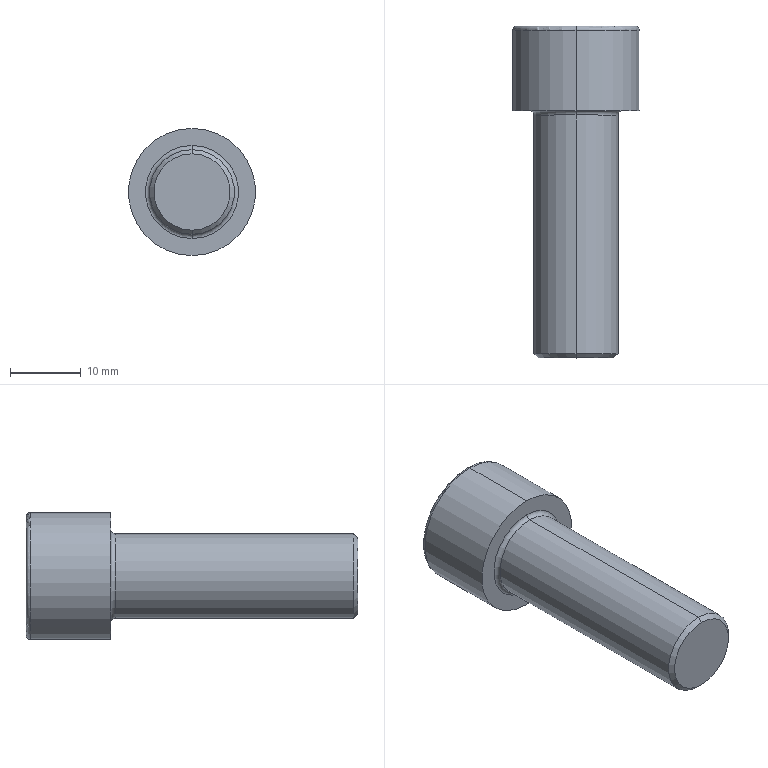Part | STEP file | 1 solid | 20 faces | box 18 x 47 x 18 mm | volume 6485 mm3 | plane 10 | torus 4 | cylinder 4 | cone 2 | commonest cylinder face diameters 12 x2 18 x2
STEP:
#1=CARTESIAN_POINT('',(0.,-35.,-5.4));
#2=VERTEX_POINT('',#1);
#3=CARTESIAN_POINT('',(0.,-35.,5.4));
#4=VERTEX_POINT('',#3);
#5=CARTESIAN_POINT('',(0.,-35.,0.));
#6=DIRECTION('',(0.,-1.,0.));
#7=DIRECTION('',(0.,0.,-1.));
#8=AXIS2_PLACEMENT_3D('',#5,#6,#7);
#9=CIRCLE('',#8,5.4);
#10=EDGE_CURVE('',#2,#4,#9,.T.);
#11=ORIENTED_EDGE('',*,*,#10,.F.);
#12=CARTESIAN_POINT('',(0.,-34.4,-6.));
#13=VERTEX_POINT('',#12);
#14=CARTESIAN_POINT('',(0.,-35.,-5.4));
#15=DIRECTION('',(0.,0.7071,-0.7071));
#16=VECTOR('',#15,1000.);
#17=LINE('',#14,#16);
#18=EDGE_CURVE('',#2,#13,#17,.T.);
#19=ORIENTED_EDGE('',*,*,#18,.T.);
#20=CARTESIAN_POINT('',(0.,-34.4,6.));
#21=VERTEX_POINT('',#20);
#22=CARTESIAN_POINT('',(0.,-34.4,0.));
#23=DIRECTION('',(0.,1.,0.));
#24=DIRECTION('',(0.,0.,-1.));
#25=AXIS2_PLACEMENT_3D('',#22,#23,#24);
#26=CIRCLE('',#25,6.);
#27=EDGE_CURVE('',#21,#13,#26,.T.);
#28=ORIENTED_EDGE('',*,*,#27,.F.);
#29=CARTESIAN_POINT('',(0.,-35.,5.4));
#30=DIRECTION('',(0.,0.7071,0.7071));
#31=VECTOR('',#30,1000.);
#32=LINE('',#29,#31);
#33=EDGE_CURVE('',#4,#21,#32,.T.);
#34=ORIENTED_EDGE('',*,*,#33,.F.);
#35=EDGE_LOOP('',(#11,#19,#28,#34));
#36=FACE_OUTER_BOUND('',#35,.T.);
#37=CARTESIAN_POINT('',(0.,-35.,0.));
#38=DIRECTION('',(0.,1.,0.));
#39=DIRECTION('',(0.,0.,1.));
#40=AXIS2_PLACEMENT_3D('',#37,#38,#39);
#41=CONICAL_SURFACE('',#40,5.4,0.7854);
#42=ADVANCED_FACE('',(#36),#41,.T.);
#43=CARTESIAN_POINT('',(0.,11.4,-9.));
#44=VERTEX_POINT('',#43);
#45=CARTESIAN_POINT('',(0.,11.4,9.));
#46=VERTEX_POINT('',#45);
#47=CARTESIAN_POINT('',(0.,11.4,0.));
#48=DIRECTION('',(0.,-1.,0.));
#49=DIRECTION('',(0.,0.,1.));
#50=AXIS2_PLACEMENT_3D('',#47,#48,#49);
#51=CIRCLE('',#50,9.);
#52=EDGE_CURVE('',#44,#46,#51,.T.);
#53=ORIENTED_EDGE('',*,*,#52,.F.);
#54=CARTESIAN_POINT('',(0.,12.,-8.4));
#55=VERTEX_POINT('',#54);
#56=CARTESIAN_POINT('',(0.,11.4,-8.4));
#57=DIRECTION('',(1.,0.,0.));
#58=DIRECTION('',(0.,0.,-1.));
#59=AXIS2_PLACEMENT_3D('',#56,#57,#58);
#60=CIRCLE('',#59,0.6);
#61=EDGE_CURVE('',#44,#55,#60,.T.);
#62=ORIENTED_EDGE('',*,*,#61,.T.);
#63=CARTESIAN_POINT('',(0.,12.,8.4));
#64=VERTEX_POINT('',#63);
#65=CARTESIAN_POINT('',(0.,12.,0.));
#66=DIRECTION('',(0.,1.,0.));
#67=DIRECTION('',(0.,0.,1.));
#68=AXIS2_PLACEMENT_3D('',#65,#66,#67);
#69=CIRCLE('',#68,8.4);
#70=EDGE_CURVE('',#64,#55,#69,.T.);
#71=ORIENTED_EDGE('',*,*,#70,.F.);
#72=CARTESIAN_POINT('',(0.,11.4,8.4));
#73=DIRECTION('',(-1.,0.,0.));
#74=DIRECTION('',(0.,0.,1.));
#75=AXIS2_PLACEMENT_3D('',#72,#73,#74);
#76=CIRCLE('',#75,0.6);
#77=EDGE_CURVE('',#46,#64,#76,.T.);
#78=ORIENTED_EDGE('',*,*,#77,.F.);
#79=EDGE_LOOP('',(#53,#62,#71,#78));
#80=FACE_OUTER_BOUND('',#79,.T.);
#81=CARTESIAN_POINT('',(0.,11.4,0.));
#82=DIRECTION('',(0.,1.,0.));
#83=DIRECTION('',(0.,0.,1.));
#84=AXIS2_PLACEMENT_3D('',#81,#82,#83);
#85=TOROIDAL_SURFACE('',#84,8.4,0.6);
#86=ADVANCED_FACE('',(#80),#85,.T.);
#87=CARTESIAN_POINT('',(0.,-0.6,6.));
#88=VERTEX_POINT('',#87);
#89=CARTESIAN_POINT('',(0.,-0.6,-6.));
#90=VERTEX_POINT('',#89);
#91=CARTESIAN_POINT('',(0.,-0.6,0.));
#92=DIRECTION('',(0.,-1.,0.));
#93=DIRECTION('',(0.,0.,-1.));
#94=AXIS2_PLACEMENT_3D('',#91,#92,#93);
#95=CIRCLE('',#94,6.);
#96=EDGE_CURVE('',#88,#90,#95,.T.);
#97=ORIENTED_EDGE('',*,*,#96,.F.);
#98=CARTESIAN_POINT('',(0.,0.,6.6));
#99=VERTEX_POINT('',#98);
#100=CARTESIAN_POINT('',(0.,-0.6,6.6));
#101=DIRECTION('',(1.,0.,0.));
#102=DIRECTION('',(0.,0.,-1.));
#103=AXIS2_PLACEMENT_3D('',#100,#101,#102);
#104=CIRCLE('',#103,0.6);
#105=EDGE_CURVE('',#88,#99,#104,.T.);
#106=ORIENTED_EDGE('',*,*,#105,.T.);
#107=CARTESIAN_POINT('',(0.,0.,-6.6));
#108=VERTEX_POINT('',#107);
#109=CARTESIAN_POINT('',(0.,0.,0.));
#110=DIRECTION('',(0.,1.,0.));
#111=DIRECTION('',(0.,0.,-1.));
#112=AXIS2_PLACEMENT_3D('',#109,#110,#111);
#113=CIRCLE('',#112,6.6);
#114=EDGE_CURVE('',#108,#99,#113,.T.);
#115=ORIENTED_EDGE('',*,*,#114,.F.);
#116=CARTESIAN_POINT('',(0.,-0.6,-6.6));
#117=DIRECTION('',(-1.,0.,0.));
#118=DIRECTION('',(0.,0.,1.));
#119=AXIS2_PLACEMENT_3D('',#116,#117,#118);
#120=CIRCLE('',#119,0.6);
#121=EDGE_CURVE('',#90,#108,#120,.T.);
#122=ORIENTED_EDGE('',*,*,#121,.F.);
#123=EDGE_LOOP('',(#97,#106,#115,#122));
#124=FACE_OUTER_BOUND('',#123,.T.);
#125=CARTESIAN_POINT('',(0.,-0.6,0.));
#126=DIRECTION('',(0.,-1.,0.));
#127=DIRECTION('',(0.,0.,-1.));
#128=AXIS2_PLACEMENT_3D('',#125,#126,#127);
#129=TOROIDAL_SURFACE('',#128,6.6,0.6);
#130=ADVANCED_FACE('',(#124),#129,.F.);
#131=CARTESIAN_POINT('',(0.,-0.6,0.));
#132=DIRECTION('',(0.,-1.,0.));
#133=DIRECTION('',(0.,0.,-1.));
#134=AXIS2_PLACEMENT_3D('',#131,#132,#133);
#135=CIRCLE('',#134,6.);
#136=EDGE_CURVE('',#90,#88,#135,.T.);
#137=ORIENTED_EDGE('',*,*,#136,.T.);
#138=CARTESIAN_POINT('',(0.,0.,6.));
#139=DIRECTION('',(0.,-1.,0.));
#140=VECTOR('',#139,1000.);
#141=LINE('',#138,#140);
#142=EDGE_CURVE('',#88,#21,#141,.T.);
#143=ORIENTED_EDGE('',*,*,#142,.T.);
#144=ORIENTED_EDGE('',*,*,#27,.T.);
#145=CARTESIAN_POINT('',(0.,0.,-6.));
#146=DIRECTION('',(0.,-1.,0.));
#147=VECTOR('',#146,1000.);
#148=LINE('',#145,#147);
#149=EDGE_CURVE('',#90,#13,#148,.T.);
#150=ORIENTED_EDGE('',*,*,#149,.F.);
#151=EDGE_LOOP('',(#137,#143,#144,#150));
#152=FACE_OUTER_BOUND('',#151,.T.);
#153=CARTESIAN_POINT('',(0.,0.,0.));
#154=DIRECTION('',(0.,-1.,0.));
#155=DIRECTION('',(0.,0.,-1.));
#156=AXIS2_PLACEMENT_3D('',#153,#154,#155);
#157=CYLINDRICAL_SURFACE('',#156,6.);
#158=ADVANCED_FACE('',(#152),#157,.T.);
#159=ORIENTED_EDGE('',*,*,#52,.T.);
#160=CARTESIAN_POINT('',(0.,0.,9.));
#161=VERTEX_POINT('',#160);
#162=CARTESIAN_POINT('',(0.,0.,9.));
#163=DIRECTION('',(0.,-1.,0.));
#164=VECTOR('',#163,1000.);
#165=LINE('',#162,#164);
#166=EDGE_CURVE('',#46,#161,#165,.T.);
#167=ORIENTED_EDGE('',*,*,#166,.T.);
#168=CARTESIAN_POINT('',(0.,0.,-9.));
#169=VERTEX_POINT('',#168);
#170=CARTESIAN_POINT('',(0.,0.,0.));
#171=DIRECTION('',(0.,-1.,0.));
#172=DIRECTION('',(0.,0.,-1.));
#173=AXIS2_PLACEMENT_3D('',#170,#171,#172);
#174=CIRCLE('',#173,9.);
#175=EDGE_CURVE('',#169,#161,#174,.T.);
#176=ORIENTED_EDGE('',*,*,#175,.F.);
#177=CARTESIAN_POINT('',(0.,0.,-9.));
#178=DIRECTION('',(0.,-1.,0.));
#179=VECTOR('',#178,1000.);
#180=LINE('',#177,#179);
#181=EDGE_CURVE('',#44,#169,#180,.T.);
#182=ORIENTED_EDGE('',*,*,#181,.F.);
#183=EDGE_LOOP('',(#159,#167,#176,#182));
#184=FACE_OUTER_BOUND('',#183,.T.);
#185=CARTESIAN_POINT('',(0.,0.,0.));
#186=DIRECTION('',(0.,-1.,0.));
#187=DIRECTION('',(0.,0.,-1.));
#188=AXIS2_PLACEMENT_3D('',#185,#186,#187);
#189=CYLINDRICAL_SURFACE('',#188,9.);
#190=ADVANCED_FACE('',(#184),#189,.T.);
#191=ORIENTED_EDGE('',*,*,#70,.T.);
#192=CARTESIAN_POINT('',(0.,12.,0.));
#193=DIRECTION('',(0.,1.,0.));
#194=DIRECTION('',(0.,0.,1.));
#195=AXIS2_PLACEMENT_3D('',#192,#193,#194);
#196=CIRCLE('',#195,8.4);
#197=EDGE_CURVE('',#55,#64,#196,.T.);
#198=ORIENTED_EDGE('',*,*,#197,.T.);
#199=EDGE_LOOP('',(#191,#198));
#200=FACE_OUTER_BOUND('',#199,.T.);
#201=CARTESIAN_POINT('',(0.,12.,-5.774));
#202=VERTEX_POINT('',#201);
#203=CARTESIAN_POINT('',(-5.,12.,-2.887));
#204=VERTEX_POINT('',#203);
#205=CARTESIAN_POINT('',(0.,12.,-5.774));
#206=DIRECTION('',(-0.866,0.,0.5));
#207=VECTOR('',#206,1000.);
#208=LINE('',#205,#207);
#209=EDGE_CURVE('',#202,#204,#208,.T.);
#210=ORIENTED_EDGE('',*,*,#209,.F.);
#211=CARTESIAN_POINT('',(5.,12.,-2.887));
#212=VERTEX_POINT('',#211);
#213=CARTESIAN_POINT('',(5.,12.,-2.887));
#214=DIRECTION('',(-0.866,0.,-0.5));
#215=VECTOR('',#214,1000.);
#216=LINE('',#213,#215);
#217=EDGE_CURVE('',#212,#202,#216,.T.);
#218=ORIENTED_EDGE('',*,*,#217,.F.);
#219=CARTESIAN_POINT('',(5.,12.,2.887));
#220=VERTEX_POINT('',#219);
#221=CARTESIAN_POINT('',(5.,12.,2.887));
#222=DIRECTION('',(0.,0.,-1.));
#223=VECTOR('',#222,1000.);
#224=LINE('',#221,#223);
#225=EDGE_CURVE('',#220,#212,#224,.T.);
#226=ORIENTED_EDGE('',*,*,#225,.F.);
#227=CARTESIAN_POINT('',(0.,12.,5.774));
#228=VERTEX_POINT('',#227);
#229=CARTESIAN_POINT('',(0.,12.,5.774));
#230=DIRECTION('',(0.866,0.,-0.5));
#231=VECTOR('',#230,1000.);
#232=LINE('',#229,#231);
#233=EDGE_CURVE('',#228,#220,#232,.T.);
#234=ORIENTED_EDGE('',*,*,#233,.F.);
#235=CARTESIAN_POINT('',(-5.,12.,2.887));
#236=VERTEX_POINT('',#235);
#237=CARTESIAN_POINT('',(-5.,12.,2.887));
#238=DIRECTION('',(0.866,0.,0.5));
#239=VECTOR('',#238,1000.);
#240=LINE('',#237,#239);
#241=EDGE_CURVE('',#236,#228,#240,.T.);
#242=ORIENTED_EDGE('',*,*,#241,.F.);
#243=CARTESIAN_POINT('',(-5.,12.,-2.887));
#244=DIRECTION('',(0.,0.,1.));
#245=VECTOR('',#244,1000.);
#246=LINE('',#243,#245);
#247=EDGE_CURVE('',#204,#236,#246,.T.);
#248=ORIENTED_EDGE('',*,*,#247,.F.);
#249=EDGE_LOOP('',(#210,#218,#226,#234,#242,#248));
#250=FACE_BOUND('',#249,.T.);
#251=CARTESIAN_POINT('',(0.,12.,0.));
#252=DIRECTION('',(0.,1.,0.));
#253=DIRECTION('',(0.,0.,1.));
#254=AXIS2_PLACEMENT_3D('',#251,#252,#253);
#255=PLANE('',#254);
#256=ADVANCED_FACE('',(#200,#250),#255,.T.);
#257=ORIENTED_EDGE('',*,*,#166,.F.);
#258=CARTESIAN_POINT('',(0.,11.4,0.));
#259=DIRECTION('',(0.,-1.,0.));
#260=DIRECTION('',(0.,0.,1.));
#261=AXIS2_PLACEMENT_3D('',#258,#259,#260);
#262=CIRCLE('',#261,9.);
#263=EDGE_CURVE('',#46,#44,#262,.T.);
#264=ORIENTED_EDGE('',*,*,#263,.T.);
#265=ORIENTED_EDGE('',*,*,#181,.T.);
#266=CARTESIAN_POINT('',(0.,0.,0.));
#267=DIRECTION('',(0.,-1.,0.));
#268=DIRECTION('',(0.,0.,-1.));
#269=AXIS2_PLACEMENT_3D('',#266,#267,#268);
#270=CIRCLE('',#269,9.);
#271=EDGE_CURVE('',#161,#169,#270,.T.);
#272=ORIENTED_EDGE('',*,*,#271,.F.);
#273=EDGE_LOOP('',(#257,#264,#265,#272));
#274=FACE_OUTER_BOUND('',#273,.T.);
#275=CARTESIAN_POINT('',(0.,0.,0.));
#276=DIRECTION('',(0.,-1.,0.));
#277=DIRECTION('',(0.,0.,-1.));
#278=AXIS2_PLACEMENT_3D('',#275,#276,#277);
#279=CYLINDRICAL_SURFACE('',#278,9.);
#280=ADVANCED_FACE('',(#274),#279,.T.);
#281=ORIENTED_EDGE('',*,*,#114,.T.);
#282=CARTESIAN_POINT('',(0.,0.,0.));
#283=DIRECTION('',(0.,1.,0.));
#284=DIRECTION('',(0.,0.,-1.));
#285=AXIS2_PLACEMENT_3D('',#282,#283,#284);
#286=CIRCLE('',#285,6.6);
#287=EDGE_CURVE('',#99,#108,#286,.T.);
#288=ORIENTED_EDGE('',*,*,#287,.T.);
#289=EDGE_LOOP('',(#281,#288));
#290=FACE_BOUND('',#289,.T.);
#291=ORIENTED_EDGE('',*,*,#175,.T.);
#292=ORIENTED_EDGE('',*,*,#271,.T.);
#293=EDGE_LOOP('',(#291,#292));
#294=FACE_OUTER_BOUND('',#293,.T.);
#295=CARTESIAN_POINT('',(9.,0.,0.));
#296=DIRECTION('',(0.,-1.,0.));
#297=DIRECTION('',(0.,0.,-1.));
#298=AXIS2_PLACEMENT_3D('',#295,#296,#297);
#299=PLANE('',#298);
#300=ADVANCED_FACE('',(#290,#294),#299,.T.);
#301=ORIENTED_EDGE('',*,*,#142,.F.);
#302=ORIENTED_EDGE('',*,*,#96,.T.);
#303=ORIENTED_EDGE('',*,*,#149,.T.);
#304=CARTESIAN_POINT('',(0.,-34.4,0.));
#305=DIRECTION('',(0.,1.,0.));
#306=DIRECTION('',(0.,0.,-1.));
#307=AXIS2_PLACEMENT_3D('',#304,#305,#306);
#308=CIRCLE('',#307,6.);
#309=EDGE_CURVE('',#13,#21,#308,.T.);
#310=ORIENTED_EDGE('',*,*,#309,.T.);
#311=EDGE_LOOP('',(#301,#302,#303,#310));
#312=FACE_OUTER_BOUND('',#311,.T.);
#313=CARTESIAN_POINT('',(0.,0.,0.));
#314=DIRECTION('',(0.,-1.,0.));
#315=DIRECTION('',(0.,0.,-1.));
#316=AXIS2_PLACEMENT_3D('',#313,#314,#315);
#317=CYLINDRICAL_SURFACE('',#316,6.);
#318=ADVANCED_FACE('',(#312),#317,.T.);
#319=CARTESIAN_POINT('',(0.,-35.,0.));
#320=DIRECTION('',(0.,-1.,0.));
#321=DIRECTION('',(0.,0.,-1.));
#322=AXIS2_PLACEMENT_3D('',#319,#320,#321);
#323=CIRCLE('',#322,5.4);
#324=EDGE_CURVE('',#4,#2,#323,.T.);
#325=ORIENTED_EDGE('',*,*,#324,.T.);
#326=ORIENTED_EDGE('',*,*,#10,.T.);
#327=EDGE_LOOP('',(#325,#326));
#328=FACE_OUTER_BOUND('',#327,.T.);
#329=CARTESIAN_POINT('',(6.,-35.,0.));
#330=DIRECTION('',(0.,-1.,0.));
#331=DIRECTION('',(0.,0.,-1.));
#332=AXIS2_PLACEMENT_3D('',#329,#330,#331);
#333=PLANE('',#332);
#334=ADVANCED_FACE('',(#328),#333,.T.);
#335=ORIENTED_EDGE('',*,*,#209,.T.);
#336=CARTESIAN_POINT('',(-5.,6.,-2.887));
#337=VERTEX_POINT('',#336);
#338=CARTESIAN_POINT('',(-5.,6.,-2.887));
#339=DIRECTION('',(0.,1.,0.));
#340=VECTOR('',#339,1000.);
#341=LINE('',#338,#340);
#342=EDGE_CURVE('',#337,#204,#341,.T.);
#343=ORIENTED_EDGE('',*,*,#342,.F.);
#344=CARTESIAN_POINT('',(0.,6.,-5.774));
#345=VERTEX_POINT('',#344);
#346=CARTESIAN_POINT('',(0.,6.,-5.774));
#347=DIRECTION('',(-0.866,0.,0.5));
#348=VECTOR('',#347,1000.);
#349=LINE('',#346,#348);
#350=EDGE_CURVE('',#345,#337,#349,.T.);
#351=ORIENTED_EDGE('',*,*,#350,.F.);
#352=CARTESIAN_POINT('',(0.,6.,-5.774));
#353=DIRECTION('',(0.,1.,0.));
#354=VECTOR('',#353,1000.);
#355=LINE('',#352,#354);
#356=EDGE_CURVE('',#345,#202,#355,.T.);
#357=ORIENTED_EDGE('',*,*,#356,.T.);
#358=EDGE_LOOP('',(#335,#343,#351,#357));
#359=FACE_OUTER_BOUND('',#358,.T.);
#360=CARTESIAN_POINT('',(0.,6.,-5.774));
#361=DIRECTION('',(-0.5,0.,-0.866));
#362=DIRECTION('',(-0.866,0.,0.5));
#363=AXIS2_PLACEMENT_3D('',#360,#361,#362);
#364=PLANE('',#363);
#365=ADVANCED_FACE('',(#359),#364,.F.);
#366=ORIENTED_EDGE('',*,*,#217,.T.);
#367=ORIENTED_EDGE('',*,*,#356,.F.);
#368=CARTESIAN_POINT('',(5.,6.,-2.887));
#369=VERTEX_POINT('',#368);
#370=CARTESIAN_POINT('',(5.,6.,-2.887));
#371=DIRECTION('',(-0.866,0.,-0.5));
#372=VECTOR('',#371,1000.);
#373=LINE('',#370,#372);
#374=EDGE_CURVE('',#369,#345,#373,.T.);
#375=ORIENTED_EDGE('',*,*,#374,.F.);
#376=CARTESIAN_POINT('',(5.,6.,-2.887));
#377=DIRECTION('',(0.,1.,0.));
#378=VECTOR('',#377,1000.);
#379=LINE('',#376,#378);
#380=EDGE_CURVE('',#369,#212,#379,.T.);
#381=ORIENTED_EDGE('',*,*,#380,.T.);
#382=EDGE_LOOP('',(#366,#367,#375,#381));
#383=FACE_OUTER_BOUND('',#382,.T.);
#384=CARTESIAN_POINT('',(5.,6.,-2.887));
#385=DIRECTION('',(0.5,0.,-0.866));
#386=DIRECTION('',(-0.866,0.,-0.5));
#387=AXIS2_PLACEMENT_3D('',#384,#385,#386);
#388=PLANE('',#387);
#389=ADVANCED_FACE('',(#383),#388,.F.);
#390=ORIENTED_EDGE('',*,*,#225,.T.);
#391=ORIENTED_EDGE('',*,*,#380,.F.);
#392=CARTESIAN_POINT('',(5.,6.,2.887));
#393=VERTEX_POINT('',#392);
#394=CARTESIAN_POINT('',(5.,6.,2.887));
#395=DIRECTION('',(0.,0.,-1.));
#396=VECTOR('',#395,1000.);
#397=LINE('',#394,#396);
#398=EDGE_CURVE('',#393,#369,#397,.T.);
#399=ORIENTED_EDGE('',*,*,#398,.F.);
#400=CARTESIAN_POINT('',(5.,6.,2.887));
#401=DIRECTION('',(0.,1.,0.));
#402=VECTOR('',#401,1000.);
#403=LINE('',#400,#402);
#404=EDGE_CURVE('',#393,#220,#403,.T.);
#405=ORIENTED_EDGE('',*,*,#404,.T.);
#406=EDGE_LOOP('',(#390,#391,#399,#405));
#407=FACE_OUTER_BOUND('',#406,.T.);
#408=CARTESIAN_POINT('',(5.,6.,2.887));
#409=DIRECTION('',(1.,0.,0.));
#410=DIRECTION('',(0.,0.,-1.));
#411=AXIS2_PLACEMENT_3D('',#408,#409,#410);
#412=PLANE('',#411);
#413=ADVANCED_FACE('',(#407),#412,.F.);
#414=ORIENTED_EDGE('',*,*,#233,.T.);
#415=ORIENTED_EDGE('',*,*,#404,.F.);
#416=CARTESIAN_POINT('',(0.,6.,5.774));
#417=VERTEX_POINT('',#416);
#418=CARTESIAN_POINT('',(0.,6.,5.774));
#419=DIRECTION('',(0.866,0.,-0.5));
#420=VECTOR('',#419,1000.);
#421=LINE('',#418,#420);
#422=EDGE_CURVE('',#417,#393,#421,.T.);
#423=ORIENTED_EDGE('',*,*,#422,.F.);
#424=CARTESIAN_POINT('',(0.,6.,5.774));
#425=DIRECTION('',(0.,1.,0.));
#426=VECTOR('',#425,1000.);
#427=LINE('',#424,#426);
#428=EDGE_CURVE('',#417,#228,#427,.T.);
#429=ORIENTED_EDGE('',*,*,#428,.T.);
#430=EDGE_LOOP('',(#414,#415,#423,#429));
#431=FACE_OUTER_BOUND('',#430,.T.);
#432=CARTESIAN_POINT('',(0.,6.,5.774));
#433=DIRECTION('',(0.5,0.,0.866));
#434=DIRECTION('',(0.866,0.,-0.5));
#435=AXIS2_PLACEMENT_3D('',#432,#433,#434);
#436=PLANE('',#435);
#437=ADVANCED_FACE('',(#431),#436,.F.);
#438=ORIENTED_EDGE('',*,*,#241,.T.);
#439=ORIENTED_EDGE('',*,*,#428,.F.);
#440=CARTESIAN_POINT('',(-5.,6.,2.887));
#441=VERTEX_POINT('',#440);
#442=CARTESIAN_POINT('',(-5.,6.,2.887));
#443=DIRECTION('',(0.866,0.,0.5));
#444=VECTOR('',#443,1000.);
#445=LINE('',#442,#444);
#446=EDGE_CURVE('',#441,#417,#445,.T.);
#447=ORIENTED_EDGE('',*,*,#446,.F.);
#448=CARTESIAN_POINT('',(-5.,6.,2.887));
#449=DIRECTION('',(0.,1.,0.));
#450=VECTOR('',#449,1000.);
#451=LINE('',#448,#450);
#452=EDGE_CURVE('',#441,#236,#451,.T.);
#453=ORIENTED_EDGE('',*,*,#452,.T.);
#454=EDGE_LOOP('',(#438,#439,#447,#453));
#455=FACE_OUTER_BOUND('',#454,.T.);
#456=CARTESIAN_POINT('',(-5.,6.,2.887));
#457=DIRECTION('',(-0.5,0.,0.866));
#458=DIRECTION('',(0.866,0.,0.5));
#459=AXIS2_PLACEMENT_3D('',#456,#457,#458);
#460=PLANE('',#459);
#461=ADVANCED_FACE('',(#455),#460,.F.);
#462=ORIENTED_EDGE('',*,*,#247,.T.);
#463=ORIENTED_EDGE('',*,*,#452,.F.);
#464=CARTESIAN_POINT('',(-5.,6.,-2.887));
#465=DIRECTION('',(0.,0.,1.));
#466=VECTOR('',#465,1000.);
#467=LINE('',#464,#466);
#468=EDGE_CURVE('',#337,#441,#467,.T.);
#469=ORIENTED_EDGE('',*,*,#468,.F.);
#470=ORIENTED_EDGE('',*,*,#342,.T.);
#471=EDGE_LOOP('',(#462,#463,#469,#470));
#472=FACE_OUTER_BOUND('',#471,.T.);
#473=CARTESIAN_POINT('',(-5.,6.,-2.887));
#474=DIRECTION('',(-1.,0.,0.));
#475=DIRECTION('',(0.,0.,1.));
#476=AXIS2_PLACEMENT_3D('',#473,#474,#475);
#477=PLANE('',#476);
#478=ADVANCED_FACE('',(#472),#477,.F.);
#479=ORIENTED_EDGE('',*,*,#350,.T.);
#480=ORIENTED_EDGE('',*,*,#468,.T.);
#481=ORIENTED_EDGE('',*,*,#446,.T.);
#482=ORIENTED_EDGE('',*,*,#422,.T.);
#483=ORIENTED_EDGE('',*,*,#398,.T.);
#484=ORIENTED_EDGE('',*,*,#374,.T.);
#485=EDGE_LOOP('',(#479,#480,#481,#482,#483,#484));
#486=FACE_OUTER_BOUND('',#485,.T.);
#487=CARTESIAN_POINT('',(0.,6.,0.));
#488=DIRECTION('',(0.,1.,0.));
#489=DIRECTION('',(0.,0.,1.));
#490=AXIS2_PLACEMENT_3D('',#487,#488,#489);
#491=PLANE('',#490);
#492=ADVANCED_FACE('',(#486),#491,.T.);
#493=ORIENTED_EDGE('',*,*,#105,.F.);
#494=ORIENTED_EDGE('',*,*,#136,.F.);
#495=ORIENTED_EDGE('',*,*,#121,.T.);
#496=ORIENTED_EDGE('',*,*,#287,.F.);
#497=EDGE_LOOP('',(#493,#494,#495,#496));
#498=FACE_OUTER_BOUND('',#497,.T.);
#499=CARTESIAN_POINT('',(0.,-0.6,0.));
#500=DIRECTION('',(0.,-1.,0.));
#501=DIRECTION('',(0.,0.,-1.));
#502=AXIS2_PLACEMENT_3D('',#499,#500,#501);
#503=TOROIDAL_SURFACE('',#502,6.6,0.6);
#504=ADVANCED_FACE('',(#498),#503,.F.);
#505=ORIENTED_EDGE('',*,*,#61,.F.);
#506=ORIENTED_EDGE('',*,*,#263,.F.);
#507=ORIENTED_EDGE('',*,*,#77,.T.);
#508=ORIENTED_EDGE('',*,*,#197,.F.);
#509=EDGE_LOOP('',(#505,#506,#507,#508));
#510=FACE_OUTER_BOUND('',#509,.T.);
#511=CARTESIAN_POINT('',(0.,11.4,0.));
#512=DIRECTION('',(0.,1.,0.));
#513=DIRECTION('',(0.,0.,1.));
#514=AXIS2_PLACEMENT_3D('',#511,#512,#513);
#515=TOROIDAL_SURFACE('',#514,8.4,0.6);
#516=ADVANCED_FACE('',(#510),#515,.T.);
#517=ORIENTED_EDGE('',*,*,#18,.F.);
#518=ORIENTED_EDGE('',*,*,#324,.F.);
#519=ORIENTED_EDGE('',*,*,#33,.T.);
#520=ORIENTED_EDGE('',*,*,#309,.F.);
#521=EDGE_LOOP('',(#517,#518,#519,#520));
#522=FACE_OUTER_BOUND('',#521,.T.);
#523=CARTESIAN_POINT('',(0.,-35.,0.));
#524=DIRECTION('',(0.,1.,0.));
#525=DIRECTION('',(0.,0.,1.));
#526=AXIS2_PLACEMENT_3D('',#523,#524,#525);
#527=CONICAL_SURFACE('',#526,5.4,0.7854);
#528=ADVANCED_FACE('',(#522),#527,.T.);
#529=CLOSED_SHELL('',(#42,#86,#130,#158,#190,#256,#280,#300,#318,#334,#365,#389,#413,#437,#461,#478,#492,#504,#516,#528));
#530=MANIFOLD_SOLID_BREP('',#529);
#531=CARTESIAN_POINT('',(0.,0.,0.));
#532=DIRECTION('',(0.,0.,1.));
#533=DIRECTION('',(1.,0.,0.));
#534=AXIS2_PLACEMENT_3D('',#531,#532,#533);
#535=(LENGTH_UNIT()NAMED_UNIT(*)SI_UNIT(.MILLI.,.METRE.));
#536=UNCERTAINTY_MEASURE_WITH_UNIT(LENGTH_MEASURE(0.00001),#535,'','');
#537=(NAMED_UNIT(*)PLANE_ANGLE_UNIT()SI_UNIT($,.RADIAN.));
#538=(NAMED_UNIT(*)SI_UNIT($,.STERADIAN.)SOLID_ANGLE_UNIT());
#539=(GEOMETRIC_REPRESENTATION_CONTEXT(3)GLOBAL_UNCERTAINTY_ASSIGNED_CONTEXT((#536))GLOBAL_UNIT_ASSIGNED_CONTEXT((#535,#537,#538))REPRESENTATION_CONTEXT('',''));
#540=ADVANCED_BREP_SHAPE_REPRESENTATION('',(#530,#534),#539);